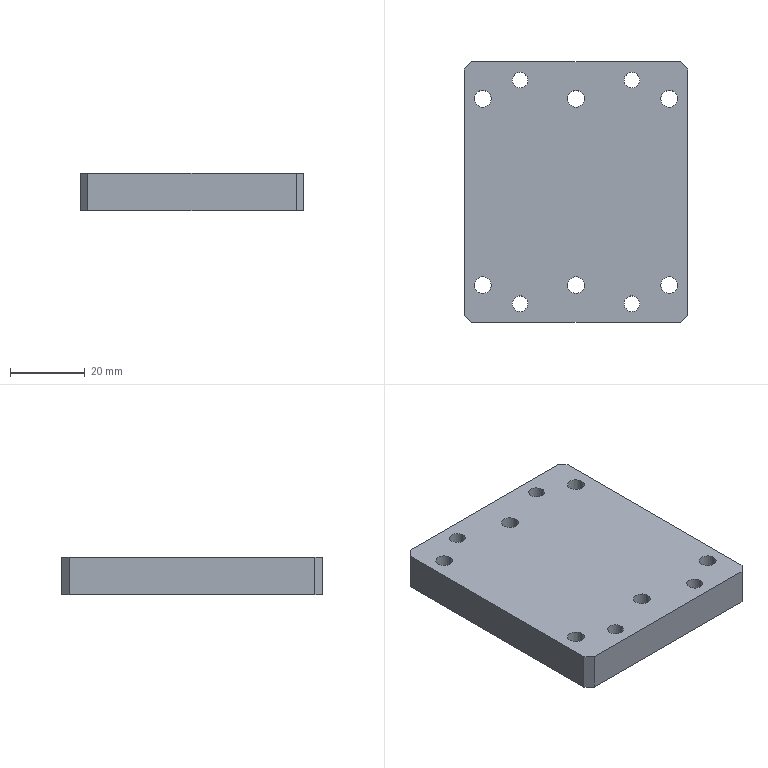Part | STEP file | 04-02-06 adjustment base plate | 1 solid | 48 faces | box 60 x 70 x 10 mm | volume 39504 mm3 | cylinder 32 | plane 16 | commonest cylinder face diameters 4.5 x12 8 x12 4.2 x8
STEP:
#1=CARTESIAN_POINT('',(12.9,-30.,10.));
#2=VERTEX_POINT('',#1);
#3=CARTESIAN_POINT('',(17.1,-30.,10.));
#4=VERTEX_POINT('',#3);
#5=CARTESIAN_POINT('',(15.,-30.,10.));
#6=DIRECTION('',(0.,0.,1.));
#7=DIRECTION('',(1.,0.,0.));
#8=AXIS2_PLACEMENT_3D('',#5,#6,#7);
#9=CIRCLE('',#8,2.1);
#10=EDGE_CURVE('',#2,#4,#9,.T.);
#11=ORIENTED_EDGE('',*,*,#10,.T.);
#12=CARTESIAN_POINT('',(17.1,-30.,0.));
#13=VERTEX_POINT('',#12);
#14=CARTESIAN_POINT('',(17.1,-30.,0.));
#15=DIRECTION('',(0.,0.,-1.));
#16=VECTOR('',#15,1000.);
#17=LINE('',#14,#16);
#18=EDGE_CURVE('',#4,#13,#17,.T.);
#19=ORIENTED_EDGE('',*,*,#18,.T.);
#20=CARTESIAN_POINT('',(12.9,-30.,0.));
#21=VERTEX_POINT('',#20);
#22=CARTESIAN_POINT('',(15.,-30.,0.));
#23=DIRECTION('',(0.,0.,-1.));
#24=DIRECTION('',(-1.,0.,0.));
#25=AXIS2_PLACEMENT_3D('',#22,#23,#24);
#26=CIRCLE('',#25,2.1);
#27=EDGE_CURVE('',#13,#21,#26,.T.);
#28=ORIENTED_EDGE('',*,*,#27,.T.);
#29=CARTESIAN_POINT('',(12.9,-30.,0.));
#30=DIRECTION('',(0.,0.,-1.));
#31=VECTOR('',#30,1000.);
#32=LINE('',#29,#31);
#33=EDGE_CURVE('',#2,#21,#32,.T.);
#34=ORIENTED_EDGE('',*,*,#33,.F.);
#35=EDGE_LOOP('',(#11,#19,#28,#34));
#36=FACE_OUTER_BOUND('',#35,.T.);
#37=CARTESIAN_POINT('',(15.,-30.,0.));
#38=DIRECTION('',(0.,0.,-1.));
#39=DIRECTION('',(-1.,0.,0.));
#40=AXIS2_PLACEMENT_3D('',#37,#38,#39);
#41=CYLINDRICAL_SURFACE('',#40,2.1);
#42=ADVANCED_FACE('',(#36),#41,.F.);
#43=CARTESIAN_POINT('',(12.9,30.,10.));
#44=VERTEX_POINT('',#43);
#45=CARTESIAN_POINT('',(17.1,30.,10.));
#46=VERTEX_POINT('',#45);
#47=CARTESIAN_POINT('',(15.,30.,10.));
#48=DIRECTION('',(0.,0.,1.));
#49=DIRECTION('',(1.,0.,0.));
#50=AXIS2_PLACEMENT_3D('',#47,#48,#49);
#51=CIRCLE('',#50,2.1);
#52=EDGE_CURVE('',#44,#46,#51,.T.);
#53=ORIENTED_EDGE('',*,*,#52,.T.);
#54=CARTESIAN_POINT('',(17.1,30.,0.));
#55=VERTEX_POINT('',#54);
#56=CARTESIAN_POINT('',(17.1,30.,0.));
#57=DIRECTION('',(0.,0.,-1.));
#58=VECTOR('',#57,1000.);
#59=LINE('',#56,#58);
#60=EDGE_CURVE('',#46,#55,#59,.T.);
#61=ORIENTED_EDGE('',*,*,#60,.T.);
#62=CARTESIAN_POINT('',(12.9,30.,0.));
#63=VERTEX_POINT('',#62);
#64=CARTESIAN_POINT('',(15.,30.,0.));
#65=DIRECTION('',(0.,0.,-1.));
#66=DIRECTION('',(-1.,0.,0.));
#67=AXIS2_PLACEMENT_3D('',#64,#65,#66);
#68=CIRCLE('',#67,2.1);
#69=EDGE_CURVE('',#55,#63,#68,.T.);
#70=ORIENTED_EDGE('',*,*,#69,.T.);
#71=CARTESIAN_POINT('',(12.9,30.,0.));
#72=DIRECTION('',(0.,0.,-1.));
#73=VECTOR('',#72,1000.);
#74=LINE('',#71,#73);
#75=EDGE_CURVE('',#44,#63,#74,.T.);
#76=ORIENTED_EDGE('',*,*,#75,.F.);
#77=EDGE_LOOP('',(#53,#61,#70,#76));
#78=FACE_OUTER_BOUND('',#77,.T.);
#79=CARTESIAN_POINT('',(15.,30.,0.));
#80=DIRECTION('',(0.,0.,-1.));
#81=DIRECTION('',(-1.,0.,0.));
#82=AXIS2_PLACEMENT_3D('',#79,#80,#81);
#83=CYLINDRICAL_SURFACE('',#82,2.1);
#84=ADVANCED_FACE('',(#78),#83,.F.);
#85=CARTESIAN_POINT('',(-17.1,30.,10.));
#86=VERTEX_POINT('',#85);
#87=CARTESIAN_POINT('',(-12.9,30.,10.));
#88=VERTEX_POINT('',#87);
#89=CARTESIAN_POINT('',(-15.,30.,10.));
#90=DIRECTION('',(0.,0.,1.));
#91=DIRECTION('',(1.,0.,0.));
#92=AXIS2_PLACEMENT_3D('',#89,#90,#91);
#93=CIRCLE('',#92,2.1);
#94=EDGE_CURVE('',#86,#88,#93,.T.);
#95=ORIENTED_EDGE('',*,*,#94,.T.);
#96=CARTESIAN_POINT('',(-12.9,30.,0.));
#97=VERTEX_POINT('',#96);
#98=CARTESIAN_POINT('',(-12.9,30.,0.));
#99=DIRECTION('',(0.,0.,-1.));
#100=VECTOR('',#99,1000.);
#101=LINE('',#98,#100);
#102=EDGE_CURVE('',#88,#97,#101,.T.);
#103=ORIENTED_EDGE('',*,*,#102,.T.);
#104=CARTESIAN_POINT('',(-17.1,30.,0.));
#105=VERTEX_POINT('',#104);
#106=CARTESIAN_POINT('',(-15.,30.,0.));
#107=DIRECTION('',(0.,0.,-1.));
#108=DIRECTION('',(-1.,0.,0.));
#109=AXIS2_PLACEMENT_3D('',#106,#107,#108);
#110=CIRCLE('',#109,2.1);
#111=EDGE_CURVE('',#97,#105,#110,.T.);
#112=ORIENTED_EDGE('',*,*,#111,.T.);
#113=CARTESIAN_POINT('',(-17.1,30.,0.));
#114=DIRECTION('',(0.,0.,-1.));
#115=VECTOR('',#114,1000.);
#116=LINE('',#113,#115);
#117=EDGE_CURVE('',#86,#105,#116,.T.);
#118=ORIENTED_EDGE('',*,*,#117,.F.);
#119=EDGE_LOOP('',(#95,#103,#112,#118));
#120=FACE_OUTER_BOUND('',#119,.T.);
#121=CARTESIAN_POINT('',(-15.,30.,0.));
#122=DIRECTION('',(0.,0.,-1.));
#123=DIRECTION('',(-1.,0.,0.));
#124=AXIS2_PLACEMENT_3D('',#121,#122,#123);
#125=CYLINDRICAL_SURFACE('',#124,2.1);
#126=ADVANCED_FACE('',(#120),#125,.F.);
#127=CARTESIAN_POINT('',(-17.1,-30.,10.));
#128=VERTEX_POINT('',#127);
#129=CARTESIAN_POINT('',(-12.9,-30.,10.));
#130=VERTEX_POINT('',#129);
#131=CARTESIAN_POINT('',(-15.,-30.,10.));
#132=DIRECTION('',(0.,0.,1.));
#133=DIRECTION('',(1.,0.,0.));
#134=AXIS2_PLACEMENT_3D('',#131,#132,#133);
#135=CIRCLE('',#134,2.1);
#136=EDGE_CURVE('',#128,#130,#135,.T.);
#137=ORIENTED_EDGE('',*,*,#136,.T.);
#138=CARTESIAN_POINT('',(-12.9,-30.,0.));
#139=VERTEX_POINT('',#138);
#140=CARTESIAN_POINT('',(-12.9,-30.,0.));
#141=DIRECTION('',(0.,0.,-1.));
#142=VECTOR('',#141,1000.);
#143=LINE('',#140,#142);
#144=EDGE_CURVE('',#130,#139,#143,.T.);
#145=ORIENTED_EDGE('',*,*,#144,.T.);
#146=CARTESIAN_POINT('',(-17.1,-30.,0.));
#147=VERTEX_POINT('',#146);
#148=CARTESIAN_POINT('',(-15.,-30.,0.));
#149=DIRECTION('',(0.,0.,-1.));
#150=DIRECTION('',(-1.,0.,0.));
#151=AXIS2_PLACEMENT_3D('',#148,#149,#150);
#152=CIRCLE('',#151,2.1);
#153=EDGE_CURVE('',#139,#147,#152,.T.);
#154=ORIENTED_EDGE('',*,*,#153,.T.);
#155=CARTESIAN_POINT('',(-17.1,-30.,0.));
#156=DIRECTION('',(0.,0.,-1.));
#157=VECTOR('',#156,1000.);
#158=LINE('',#155,#157);
#159=EDGE_CURVE('',#128,#147,#158,.T.);
#160=ORIENTED_EDGE('',*,*,#159,.F.);
#161=EDGE_LOOP('',(#137,#145,#154,#160));
#162=FACE_OUTER_BOUND('',#161,.T.);
#163=CARTESIAN_POINT('',(-15.,-30.,0.));
#164=DIRECTION('',(0.,0.,-1.));
#165=DIRECTION('',(-1.,0.,0.));
#166=AXIS2_PLACEMENT_3D('',#163,#164,#165);
#167=CYLINDRICAL_SURFACE('',#166,2.1);
#168=ADVANCED_FACE('',(#162),#167,.F.);
#169=CARTESIAN_POINT('',(29.,25.,4.4));
#170=VERTEX_POINT('',#169);
#171=CARTESIAN_POINT('',(21.,25.,4.4));
#172=VERTEX_POINT('',#171);
#173=CARTESIAN_POINT('',(25.,25.,4.4));
#174=DIRECTION('',(0.,0.,-1.));
#175=DIRECTION('',(-1.,0.,0.));
#176=AXIS2_PLACEMENT_3D('',#173,#174,#175);
#177=CIRCLE('',#176,4.);
#178=EDGE_CURVE('',#170,#172,#177,.T.);
#179=ORIENTED_EDGE('',*,*,#178,.F.);
#180=CARTESIAN_POINT('',(29.,25.,0.));
#181=VERTEX_POINT('',#180);
#182=CARTESIAN_POINT('',(29.,25.,0.));
#183=DIRECTION('',(0.,0.,-1.));
#184=VECTOR('',#183,1000.);
#185=LINE('',#182,#184);
#186=EDGE_CURVE('',#170,#181,#185,.T.);
#187=ORIENTED_EDGE('',*,*,#186,.T.);
#188=CARTESIAN_POINT('',(21.,25.,0.));
#189=VERTEX_POINT('',#188);
#190=CARTESIAN_POINT('',(25.,25.,0.));
#191=DIRECTION('',(0.,0.,-1.));
#192=DIRECTION('',(-1.,0.,0.));
#193=AXIS2_PLACEMENT_3D('',#190,#191,#192);
#194=CIRCLE('',#193,4.);
#195=EDGE_CURVE('',#181,#189,#194,.T.);
#196=ORIENTED_EDGE('',*,*,#195,.T.);
#197=CARTESIAN_POINT('',(21.,25.,0.));
#198=DIRECTION('',(0.,0.,-1.));
#199=VECTOR('',#198,1000.);
#200=LINE('',#197,#199);
#201=EDGE_CURVE('',#172,#189,#200,.T.);
#202=ORIENTED_EDGE('',*,*,#201,.F.);
#203=EDGE_LOOP('',(#179,#187,#196,#202));
#204=FACE_OUTER_BOUND('',#203,.T.);
#205=CARTESIAN_POINT('',(25.,25.,0.));
#206=DIRECTION('',(0.,0.,-1.));
#207=DIRECTION('',(-1.,0.,0.));
#208=AXIS2_PLACEMENT_3D('',#205,#206,#207);
#209=CYLINDRICAL_SURFACE('',#208,4.);
#210=ADVANCED_FACE('',(#204),#209,.F.);
#211=CARTESIAN_POINT('',(27.25,25.,10.));
#212=VERTEX_POINT('',#211);
#213=CARTESIAN_POINT('',(22.75,25.,10.));
#214=VERTEX_POINT('',#213);
#215=CARTESIAN_POINT('',(25.,25.,10.));
#216=DIRECTION('',(0.,0.,-1.));
#217=DIRECTION('',(-1.,0.,0.));
#218=AXIS2_PLACEMENT_3D('',#215,#216,#217);
#219=CIRCLE('',#218,2.25);
#220=EDGE_CURVE('',#212,#214,#219,.T.);
#221=ORIENTED_EDGE('',*,*,#220,.F.);
#222=CARTESIAN_POINT('',(27.25,25.,4.4));
#223=VERTEX_POINT('',#222);
#224=CARTESIAN_POINT('',(27.25,25.,0.));
#225=DIRECTION('',(0.,0.,-1.));
#226=VECTOR('',#225,1000.);
#227=LINE('',#224,#226);
#228=EDGE_CURVE('',#212,#223,#227,.T.);
#229=ORIENTED_EDGE('',*,*,#228,.T.);
#230=CARTESIAN_POINT('',(22.75,25.,4.4));
#231=VERTEX_POINT('',#230);
#232=CARTESIAN_POINT('',(25.,25.,4.4));
#233=DIRECTION('',(0.,0.,-1.));
#234=DIRECTION('',(-1.,0.,0.));
#235=AXIS2_PLACEMENT_3D('',#232,#233,#234);
#236=CIRCLE('',#235,2.25);
#237=EDGE_CURVE('',#223,#231,#236,.T.);
#238=ORIENTED_EDGE('',*,*,#237,.T.);
#239=CARTESIAN_POINT('',(22.75,25.,0.));
#240=DIRECTION('',(0.,0.,-1.));
#241=VECTOR('',#240,1000.);
#242=LINE('',#239,#241);
#243=EDGE_CURVE('',#214,#231,#242,.T.);
#244=ORIENTED_EDGE('',*,*,#243,.F.);
#245=EDGE_LOOP('',(#221,#229,#238,#244));
#246=FACE_OUTER_BOUND('',#245,.T.);
#247=CARTESIAN_POINT('',(25.,25.,0.));
#248=DIRECTION('',(0.,0.,-1.));
#249=DIRECTION('',(-1.,0.,0.));
#250=AXIS2_PLACEMENT_3D('',#247,#248,#249);
#251=CYLINDRICAL_SURFACE('',#250,2.25);
#252=ADVANCED_FACE('',(#246),#251,.F.);
#253=CARTESIAN_POINT('',(29.,-25.,4.4));
#254=VERTEX_POINT('',#253);
#255=CARTESIAN_POINT('',(21.,-25.,4.4));
#256=VERTEX_POINT('',#255);
#257=CARTESIAN_POINT('',(25.,-25.,4.4));
#258=DIRECTION('',(0.,0.,-1.));
#259=DIRECTION('',(-1.,0.,0.));
#260=AXIS2_PLACEMENT_3D('',#257,#258,#259);
#261=CIRCLE('',#260,4.);
#262=EDGE_CURVE('',#254,#256,#261,.T.);
#263=ORIENTED_EDGE('',*,*,#262,.F.);
#264=CARTESIAN_POINT('',(29.,-25.,0.));
#265=VERTEX_POINT('',#264);
#266=CARTESIAN_POINT('',(29.,-25.,0.));
#267=DIRECTION('',(0.,0.,-1.));
#268=VECTOR('',#267,1000.);
#269=LINE('',#266,#268);
#270=EDGE_CURVE('',#254,#265,#269,.T.);
#271=ORIENTED_EDGE('',*,*,#270,.T.);
#272=CARTESIAN_POINT('',(21.,-25.,0.));
#273=VERTEX_POINT('',#272);
#274=CARTESIAN_POINT('',(25.,-25.,0.));
#275=DIRECTION('',(0.,0.,-1.));
#276=DIRECTION('',(-1.,0.,0.));
#277=AXIS2_PLACEMENT_3D('',#274,#275,#276);
#278=CIRCLE('',#277,4.);
#279=EDGE_CURVE('',#265,#273,#278,.T.);
#280=ORIENTED_EDGE('',*,*,#279,.T.);
#281=CARTESIAN_POINT('',(21.,-25.,0.));
#282=DIRECTION('',(0.,0.,-1.));
#283=VECTOR('',#282,1000.);
#284=LINE('',#281,#283);
#285=EDGE_CURVE('',#256,#273,#284,.T.);
#286=ORIENTED_EDGE('',*,*,#285,.F.);
#287=EDGE_LOOP('',(#263,#271,#280,#286));
#288=FACE_OUTER_BOUND('',#287,.T.);
#289=CARTESIAN_POINT('',(25.,-25.,0.));
#290=DIRECTION('',(0.,0.,-1.));
#291=DIRECTION('',(-1.,0.,0.));
#292=AXIS2_PLACEMENT_3D('',#289,#290,#291);
#293=CYLINDRICAL_SURFACE('',#292,4.);
#294=ADVANCED_FACE('',(#288),#293,.F.);
#295=CARTESIAN_POINT('',(27.25,-25.,10.));
#296=VERTEX_POINT('',#295);
#297=CARTESIAN_POINT('',(22.75,-25.,10.));
#298=VERTEX_POINT('',#297);
#299=CARTESIAN_POINT('',(25.,-25.,10.));
#300=DIRECTION('',(0.,0.,-1.));
#301=DIRECTION('',(-1.,0.,0.));
#302=AXIS2_PLACEMENT_3D('',#299,#300,#301);
#303=CIRCLE('',#302,2.25);
#304=EDGE_CURVE('',#296,#298,#303,.T.);
#305=ORIENTED_EDGE('',*,*,#304,.F.);
#306=CARTESIAN_POINT('',(27.25,-25.,4.4));
#307=VERTEX_POINT('',#306);
#308=CARTESIAN_POINT('',(27.25,-25.,0.));
#309=DIRECTION('',(0.,0.,-1.));
#310=VECTOR('',#309,1000.);
#311=LINE('',#308,#310);
#312=EDGE_CURVE('',#296,#307,#311,.T.);
#313=ORIENTED_EDGE('',*,*,#312,.T.);
#314=CARTESIAN_POINT('',(22.75,-25.,4.4));
#315=VERTEX_POINT('',#314);
#316=CARTESIAN_POINT('',(25.,-25.,4.4));
#317=DIRECTION('',(0.,0.,-1.));
#318=DIRECTION('',(-1.,0.,0.));
#319=AXIS2_PLACEMENT_3D('',#316,#317,#318);
#320=CIRCLE('',#319,2.25);
#321=EDGE_CURVE('',#307,#315,#320,.T.);
#322=ORIENTED_EDGE('',*,*,#321,.T.);
#323=CARTESIAN_POINT('',(22.75,-25.,0.));
#324=DIRECTION('',(0.,0.,-1.));
#325=VECTOR('',#324,1000.);
#326=LINE('',#323,#325);
#327=EDGE_CURVE('',#298,#315,#326,.T.);
#328=ORIENTED_EDGE('',*,*,#327,.F.);
#329=EDGE_LOOP('',(#305,#313,#322,#328));
#330=FACE_OUTER_BOUND('',#329,.T.);
#331=CARTESIAN_POINT('',(25.,-25.,0.));
#332=DIRECTION('',(0.,0.,-1.));
#333=DIRECTION('',(-1.,0.,0.));
#334=AXIS2_PLACEMENT_3D('',#331,#332,#333);
#335=CYLINDRICAL_SURFACE('',#334,2.25);
#336=ADVANCED_FACE('',(#330),#335,.F.);
#337=CARTESIAN_POINT('',(4.,-25.,4.4));
#338=VERTEX_POINT('',#337);
#339=CARTESIAN_POINT('',(-4.,-25.,4.4));
#340=VERTEX_POINT('',#339);
#341=CARTESIAN_POINT('',(0.,-25.,4.4));
#342=DIRECTION('',(0.,0.,-1.));
#343=DIRECTION('',(-1.,0.,0.));
#344=AXIS2_PLACEMENT_3D('',#341,#342,#343);
#345=CIRCLE('',#344,4.);
#346=EDGE_CURVE('',#338,#340,#345,.T.);
#347=ORIENTED_EDGE('',*,*,#346,.F.);
#348=CARTESIAN_POINT('',(4.,-25.,0.));
#349=VERTEX_POINT('',#348);
#350=CARTESIAN_POINT('',(4.,-25.,0.));
#351=DIRECTION('',(0.,0.,-1.));
#352=VECTOR('',#351,1000.);
#353=LINE('',#350,#352);
#354=EDGE_CURVE('',#338,#349,#353,.T.);
#355=ORIENTED_EDGE('',*,*,#354,.T.);
#356=CARTESIAN_POINT('',(-4.,-25.,0.));
#357=VERTEX_POINT('',#356);
#358=CARTESIAN_POINT('',(0.,-25.,0.));
#359=DIRECTION('',(0.,0.,-1.));
#360=DIRECTION('',(-1.,0.,0.));
#361=AXIS2_PLACEMENT_3D('',#358,#359,#360);
#362=CIRCLE('',#361,4.);
#363=EDGE_CURVE('',#349,#357,#362,.T.);
#364=ORIENTED_EDGE('',*,*,#363,.T.);
#365=CARTESIAN_POINT('',(-4.,-25.,0.));
#366=DIRECTION('',(0.,0.,-1.));
#367=VECTOR('',#366,1000.);
#368=LINE('',#365,#367);
#369=EDGE_CURVE('',#340,#357,#368,.T.);
#370=ORIENTED_EDGE('',*,*,#369,.F.);
#371=EDGE_LOOP('',(#347,#355,#364,#370));
#372=FACE_OUTER_BOUND('',#371,.T.);
#373=CARTESIAN_POINT('',(0.,-25.,0.));
#374=DIRECTION('',(0.,0.,-1.));
#375=DIRECTION('',(-1.,0.,0.));
#376=AXIS2_PLACEMENT_3D('',#373,#374,#375);
#377=CYLINDRICAL_SURFACE('',#376,4.);
#378=ADVANCED_FACE('',(#372),#377,.F.);
#379=CARTESIAN_POINT('',(2.25,-25.,10.));
#380=VERTEX_POINT('',#379);
#381=CARTESIAN_POINT('',(-2.25,-25.,10.));
#382=VERTEX_POINT('',#381);
#383=CARTESIAN_POINT('',(0.,-25.,10.));
#384=DIRECTION('',(0.,0.,-1.));
#385=DIRECTION('',(-1.,0.,0.));
#386=AXIS2_PLACEMENT_3D('',#383,#384,#385);
#387=CIRCLE('',#386,2.25);
#388=EDGE_CURVE('',#380,#382,#387,.T.);
#389=ORIENTED_EDGE('',*,*,#388,.F.);
#390=CARTESIAN_POINT('',(2.25,-25.,4.4));
#391=VERTEX_POINT('',#390);
#392=CARTESIAN_POINT('',(2.25,-25.,0.));
#393=DIRECTION('',(0.,0.,-1.));
#394=VECTOR('',#393,1000.);
#395=LINE('',#392,#394);
#396=EDGE_CURVE('',#380,#391,#395,.T.);
#397=ORIENTED_EDGE('',*,*,#396,.T.);
#398=CARTESIAN_POINT('',(-2.25,-25.,4.4));
#399=VERTEX_POINT('',#398);
#400=CARTESIAN_POINT('',(0.,-25.,4.4));
#401=DIRECTION('',(0.,0.,-1.));
#402=DIRECTION('',(-1.,0.,0.));
#403=AXIS2_PLACEMENT_3D('',#400,#401,#402);
#404=CIRCLE('',#403,2.25);
#405=EDGE_CURVE('',#391,#399,#404,.T.);
#406=ORIENTED_EDGE('',*,*,#405,.T.);
#407=CARTESIAN_POINT('',(-2.25,-25.,0.));
#408=DIRECTION('',(0.,0.,-1.));
#409=VECTOR('',#408,1000.);
#410=LINE('',#407,#409);
#411=EDGE_CURVE('',#382,#399,#410,.T.);
#412=ORIENTED_EDGE('',*,*,#411,.F.);
#413=EDGE_LOOP('',(#389,#397,#406,#412));
#414=FACE_OUTER_BOUND('',#413,.T.);
#415=CARTESIAN_POINT('',(0.,-25.,0.));
#416=DIRECTION('',(0.,0.,-1.));
#417=DIRECTION('',(-1.,0.,0.));
#418=AXIS2_PLACEMENT_3D('',#415,#416,#417);
#419=CYLINDRICAL_SURFACE('',#418,2.25);
#420=ADVANCED_FACE('',(#414),#419,.F.);
#421=CARTESIAN_POINT('',(-21.,-25.,4.4));
#422=VERTEX_POINT('',#421);
#423=CARTESIAN_POINT('',(-29.,-25.,4.4));
#424=VERTEX_POINT('',#423);
#425=CARTESIAN_POINT('',(-25.,-25.,4.4));
#426=DIRECTION('',(0.,0.,-1.));
#427=DIRECTION('',(-1.,0.,0.));
#428=AXIS2_PLACEMENT_3D('',#425,#426,#427);
#429=CIRCLE('',#428,4.);
#430=EDGE_CURVE('',#422,#424,#429,.T.);
#431=ORIENTED_EDGE('',*,*,#430,.F.);
#432=CARTESIAN_POINT('',(-21.,-25.,0.));
#433=VERTEX_POINT('',#432);
#434=CARTESIAN_POINT('',(-21.,-25.,0.));
#435=DIRECTION('',(0.,0.,-1.));
#436=VECTOR('',#435,1000.);
#437=LINE('',#434,#436);
#438=EDGE_CURVE('',#422,#433,#437,.T.);
#439=ORIENTED_EDGE('',*,*,#438,.T.);
#440=CARTESIAN_POINT('',(-29.,-25.,0.));
#441=VERTEX_POINT('',#440);
#442=CARTESIAN_POINT('',(-25.,-25.,0.));
#443=DIRECTION('',(0.,0.,-1.));
#444=DIRECTION('',(-1.,0.,0.));
#445=AXIS2_PLACEMENT_3D('',#442,#443,#444);
#446=CIRCLE('',#445,4.);
#447=EDGE_CURVE('',#433,#441,#446,.T.);
#448=ORIENTED_EDGE('',*,*,#447,.T.);
#449=CARTESIAN_POINT('',(-29.,-25.,0.));
#450=DIRECTION('',(0.,0.,-1.));
#451=VECTOR('',#450,1000.);
#452=LINE('',#449,#451);
#453=EDGE_CURVE('',#424,#441,#452,.T.);
#454=ORIENTED_EDGE('',*,*,#453,.F.);
#455=EDGE_LOOP('',(#431,#439,#448,#454));
#456=FACE_OUTER_BOUND('',#455,.T.);
#457=CARTESIAN_POINT('',(-25.,-25.,0.));
#458=DIRECTION('',(0.,0.,-1.));
#459=DIRECTION('',(-1.,0.,0.));
#460=AXIS2_PLACEMENT_3D('',#457,#458,#459);
#461=CYLINDRICAL_SURFACE('',#460,4.);
#462=ADVANCED_FACE('',(#456),#461,.F.);
#463=CARTESIAN_POINT('',(-22.75,-25.,10.));
#464=VERTEX_POINT('',#463);
#465=CARTESIAN_POINT('',(-27.25,-25.,10.));
#466=VERTEX_POINT('',#465);
#467=CARTESIAN_POINT('',(-25.,-25.,10.));
#468=DIRECTION('',(0.,0.,-1.));
#469=DIRECTION('',(-1.,0.,0.));
#470=AXIS2_PLACEMENT_3D('',#467,#468,#469);
#471=CIRCLE('',#470,2.25);
#472=EDGE_CURVE('',#464,#466,#471,.T.);
#473=ORIENTED_EDGE('',*,*,#472,.F.);
#474=CARTESIAN_POINT('',(-22.75,-25.,4.4));
#475=VERTEX_POINT('',#474);
#476=CARTESIAN_POINT('',(-22.75,-25.,0.));
#477=DIRECTION('',(0.,0.,-1.));
#478=VECTOR('',#477,1000.);
#479=LINE('',#476,#478);
#480=EDGE_CURVE('',#464,#475,#479,.T.);
#481=ORIENTED_EDGE('',*,*,#480,.T.);
#482=CARTESIAN_POINT('',(-27.25,-25.,4.4));
#483=VERTEX_POINT('',#482);
#484=CARTESIAN_POINT('',(-25.,-25.,4.4));
#485=DIRECTION('',(0.,0.,-1.));
#486=DIRECTION('',(-1.,0.,0.));
#487=AXIS2_PLACEMENT_3D('',#484,#485,#486);
#488=CIRCLE('',#487,2.25);
#489=EDGE_CURVE('',#475,#483,#488,.T.);
#490=ORIENTED_EDGE('',*,*,#489,.T.);
#491=CARTESIAN_POINT('',(-27.25,-25.,0.));
#492=DIRECTION('',(0.,0.,-1.));
#493=VECTOR('',#492,1000.);
#494=LINE('',#491,#493);
#495=EDGE_CURVE('',#466,#483,#494,.T.);
#496=ORIENTED_EDGE('',*,*,#495,.F.);
#497=EDGE_LOOP('',(#473,#481,#490,#496));
#498=FACE_OUTER_BOUND('',#497,.T.);
#499=CARTESIAN_POINT('',(-25.,-25.,0.));
#500=DIRECTION('',(0.,0.,-1.));
#501=DIRECTION('',(-1.,0.,0.));
#502=AXIS2_PLACEMENT_3D('',#499,#500,#501);
#503=CYLINDRICAL_SURFACE('',#502,2.25);
#504=ADVANCED_FACE('',(#498),#503,.F.);
#505=CARTESIAN_POINT('',(-21.,25.,4.4));
#506=VERTEX_POINT('',#505);
#507=CARTESIAN_POINT('',(-29.,25.,4.4));
#508=VERTEX_POINT('',#507);
#509=CARTESIAN_POINT('',(-25.,25.,4.4));
#510=DIRECTION('',(0.,0.,-1.));
#511=DIRECTION('',(-1.,0.,0.));
#512=AXIS2_PLACEMENT_3D('',#509,#510,#511);
#513=CIRCLE('',#512,4.);
#514=EDGE_CURVE('',#506,#508,#513,.T.);
#515=ORIENTED_EDGE('',*,*,#514,.F.);
#516=CARTESIAN_POINT('',(-21.,25.,0.));
#517=VERTEX_POINT('',#516);
#518=CARTESIAN_POINT('',(-21.,25.,0.));
#519=DIRECTION('',(0.,0.,-1.));
#520=VECTOR('',#519,1000.);
#521=LINE('',#518,#520);
#522=EDGE_CURVE('',#506,#517,#521,.T.);
#523=ORIENTED_EDGE('',*,*,#522,.T.);
#524=CARTESIAN_POINT('',(-29.,25.,0.));
#525=VERTEX_POINT('',#524);
#526=CARTESIAN_POINT('',(-25.,25.,0.));
#527=DIRECTION('',(0.,0.,-1.));
#528=DIRECTION('',(-1.,0.,0.));
#529=AXIS2_PLACEMENT_3D('',#526,#527,#528);
#530=CIRCLE('',#529,4.);
#531=EDGE_CURVE('',#517,#525,#530,.T.);
#532=ORIENTED_EDGE('',*,*,#531,.T.);
#533=CARTESIAN_POINT('',(-29.,25.,0.));
#534=DIRECTION('',(0.,0.,-1.));
#535=VECTOR('',#534,1000.);
#536=LINE('',#533,#535);
#537=EDGE_CURVE('',#508,#525,#536,.T.);
#538=ORIENTED_EDGE('',*,*,#537,.F.);
#539=EDGE_LOOP('',(#515,#523,#532,#538));
#540=FACE_OUTER_BOUND('',#539,.T.);
#541=CARTESIAN_POINT('',(-25.,25.,0.));
#542=DIRECTION('',(0.,0.,-1.));
#543=DIRECTION('',(-1.,0.,0.));
#544=AXIS2_PLACEMENT_3D('',#541,#542,#543);
#545=CYLINDRICAL_SURFACE('',#544,4.);
#546=ADVANCED_FACE('',(#540),#545,.F.);
#547=CARTESIAN_POINT('',(-22.75,25.,10.));
#548=VERTEX_POINT('',#547);
#549=CARTESIAN_POINT('',(-27.25,25.,10.));
#550=VERTEX_POINT('',#549);
#551=CARTESIAN_POINT('',(-25.,25.,10.));
#552=DIRECTION('',(0.,0.,-1.));
#553=DIRECTION('',(-1.,0.,0.));
#554=AXIS2_PLACEMENT_3D('',#551,#552,#553);
#555=CIRCLE('',#554,2.25);
#556=EDGE_CURVE('',#548,#550,#555,.T.);
#557=ORIENTED_EDGE('',*,*,#556,.F.);
#558=CARTESIAN_POINT('',(-22.75,25.,4.4));
#559=VERTEX_POINT('',#558);
#560=CARTESIAN_POINT('',(-22.75,25.,0.));
#561=DIRECTION('',(0.,0.,-1.));
#562=VECTOR('',#561,1000.);
#563=LINE('',#560,#562);
#564=EDGE_CURVE('',#548,#559,#563,.T.);
#565=ORIENTED_EDGE('',*,*,#564,.T.);
#566=CARTESIAN_POINT('',(-27.25,25.,4.4));
#567=VERTEX_POINT('',#566);
#568=CARTESIAN_POINT('',(-25.,25.,4.4));
#569=DIRECTION('',(0.,0.,-1.));
#570=DIRECTION('',(-1.,0.,0.));
#571=AXIS2_PLACEMENT_3D('',#568,#569,#570);
#572=CIRCLE('',#571,2.25);
#573=EDGE_CURVE('',#559,#567,#572,.T.);
#574=ORIENTED_EDGE('',*,*,#573,.T.);
#575=CARTESIAN_POINT('',(-27.25,25.,0.));
#576=DIRECTION('',(0.,0.,-1.));
#577=VECTOR('',#576,1000.);
#578=LINE('',#575,#577);
#579=EDGE_CURVE('',#550,#567,#578,.T.);
#580=ORIENTED_EDGE('',*,*,#579,.F.);
#581=EDGE_LOOP('',(#557,#565,#574,#580));
#582=FACE_OUTER_BOUND('',#581,.T.);
#583=CARTESIAN_POINT('',(-25.,25.,0.));
#584=DIRECTION('',(0.,0.,-1.));
#585=DIRECTION('',(-1.,0.,0.));
#586=AXIS2_PLACEMENT_3D('',#583,#584,#585);
#587=CYLINDRICAL_SURFACE('',#586,2.25);
#588=ADVANCED_FACE('',(#582),#587,.F.);
#589=CARTESIAN_POINT('',(4.,25.,4.4));
#590=VERTEX_POINT('',#589);
#591=CARTESIAN_POINT('',(-4.,25.,4.4));
#592=VERTEX_POINT('',#591);
#593=CARTESIAN_POINT('',(0.,25.,4.4));
#594=DIRECTION('',(0.,0.,-1.));
#595=DIRECTION('',(-1.,0.,0.));
#596=AXIS2_PLACEMENT_3D('',#593,#594,#595);
#597=CIRCLE('',#596,4.);
#598=EDGE_CURVE('',#590,#592,#597,.T.);
#599=ORIENTED_EDGE('',*,*,#598,.F.);
#600=CARTESIAN_POINT('',(4.,25.,0.));
#601=VERTEX_POINT('',#600);
#602=CARTESIAN_POINT('',(4.,25.,0.));
#603=DIRECTION('',(0.,0.,-1.));
#604=VECTOR('',#603,1000.);
#605=LINE('',#602,#604);
#606=EDGE_CURVE('',#590,#601,#605,.T.);
#607=ORIENTED_EDGE('',*,*,#606,.T.);
#608=CARTESIAN_POINT('',(-4.,25.,0.));
#609=VERTEX_POINT('',#608);
#610=CARTESIAN_POINT('',(0.,25.,0.));
#611=DIRECTION('',(0.,0.,-1.));
#612=DIRECTION('',(-1.,0.,0.));
#613=AXIS2_PLACEMENT_3D('',#610,#611,#612);
#614=CIRCLE('',#613,4.);
#615=EDGE_CURVE('',#601,#609,#614,.T.);
#616=ORIENTED_EDGE('',*,*,#615,.T.);
#617=CARTESIAN_POINT('',(-4.,25.,0.));
#618=DIRECTION('',(0.,0.,-1.));
#619=VECTOR('',#618,1000.);
#620=LINE('',#617,#619);
#621=EDGE_CURVE('',#592,#609,#620,.T.);
#622=ORIENTED_EDGE('',*,*,#621,.F.);
#623=EDGE_LOOP('',(#599,#607,#616,#622));
#624=FACE_OUTER_BOUND('',#623,.T.);
#625=CARTESIAN_POINT('',(0.,25.,0.));
#626=DIRECTION('',(0.,0.,-1.));
#627=DIRECTION('',(-1.,0.,0.));
#628=AXIS2_PLACEMENT_3D('',#625,#626,#627);
#629=CYLINDRICAL_SURFACE('',#628,4.);
#630=ADVANCED_FACE('',(#624),#629,.F.);
#631=CARTESIAN_POINT('',(2.25,25.,10.));
#632=VERTEX_POINT('',#631);
#633=CARTESIAN_POINT('',(-2.25,25.,10.));
#634=VERTEX_POINT('',#633);
#635=CARTESIAN_POINT('',(0.,25.,10.));
#636=DIRECTION('',(0.,0.,-1.));
#637=DIRECTION('',(-1.,0.,0.));
#638=AXIS2_PLACEMENT_3D('',#635,#636,#637);
#639=CIRCLE('',#638,2.25);
#640=EDGE_CURVE('',#632,#634,#639,.T.);
#641=ORIENTED_EDGE('',*,*,#640,.F.);
#642=CARTESIAN_POINT('',(2.25,25.,4.4));
#643=VERTEX_POINT('',#642);
#644=CARTESIAN_POINT('',(2.25,25.,0.));
#645=DIRECTION('',(0.,0.,-1.));
#646=VECTOR('',#645,1000.);
#647=LINE('',#644,#646);
#648=EDGE_CURVE('',#632,#643,#647,.T.);
#649=ORIENTED_EDGE('',*,*,#648,.T.);
#650=CARTESIAN_POINT('',(-2.25,25.,4.4));
#651=VERTEX_POINT('',#650);
#652=CARTESIAN_POINT('',(0.,25.,4.4));
#653=DIRECTION('',(0.,0.,-1.));
#654=DIRECTION('',(-1.,0.,0.));
#655=AXIS2_PLACEMENT_3D('',#652,#653,#654);
#656=CIRCLE('',#655,2.25);
#657=EDGE_CURVE('',#643,#651,#656,.T.);
#658=ORIENTED_EDGE('',*,*,#657,.T.);
#659=CARTESIAN_POINT('',(-2.25,25.,0.));
#660=DIRECTION('',(0.,0.,-1.));
#661=VECTOR('',#660,1000.);
#662=LINE('',#659,#661);
#663=EDGE_CURVE('',#634,#651,#662,.T.);
#664=ORIENTED_EDGE('',*,*,#663,.F.);
#665=EDGE_LOOP('',(#641,#649,#658,#664));
#666=FACE_OUTER_BOUND('',#665,.T.);
#667=CARTESIAN_POINT('',(0.,25.,0.));
#668=DIRECTION('',(0.,0.,-1.));
#669=DIRECTION('',(-1.,0.,0.));
#670=AXIS2_PLACEMENT_3D('',#667,#668,#669);
#671=CYLINDRICAL_SURFACE('',#670,2.25);
#672=ADVANCED_FACE('',(#666),#671,.F.);
#673=CARTESIAN_POINT('',(28.,35.,0.));
#674=VERTEX_POINT('',#673);
#675=CARTESIAN_POINT('',(-28.,35.,0.));
#676=VERTEX_POINT('',#675);
#677=CARTESIAN_POINT('',(-30.,35.,0.));
#678=DIRECTION('',(-1.,0.,0.));
#679=VECTOR('',#678,1000.);
#680=LINE('',#677,#679);
#681=EDGE_CURVE('',#674,#676,#680,.T.);
#682=ORIENTED_EDGE('',*,*,#681,.F.);
#683=CARTESIAN_POINT('',(30.,33.,0.));
#684=VERTEX_POINT('',#683);
#685=CARTESIAN_POINT('',(28.,35.,0.));
#686=DIRECTION('',(0.7071,-0.7071,0.));
#687=VECTOR('',#686,1000.);
#688=LINE('',#685,#687);
#689=EDGE_CURVE('',#674,#684,#688,.T.);
#690=ORIENTED_EDGE('',*,*,#689,.T.);
#691=CARTESIAN_POINT('',(30.,-33.,0.));
#692=VERTEX_POINT('',#691);
#693=CARTESIAN_POINT('',(30.,35.,0.));
#694=DIRECTION('',(0.,1.,0.));
#695=VECTOR('',#694,1000.);
#696=LINE('',#693,#695);
#697=EDGE_CURVE('',#692,#684,#696,.T.);
#698=ORIENTED_EDGE('',*,*,#697,.F.);
#699=CARTESIAN_POINT('',(28.,-35.,0.));
#700=VERTEX_POINT('',#699);
#701=CARTESIAN_POINT('',(30.,-33.,0.));
#702=DIRECTION('',(-0.7071,-0.7071,0.));
#703=VECTOR('',#702,1000.);
#704=LINE('',#701,#703);
#705=EDGE_CURVE('',#692,#700,#704,.T.);
#706=ORIENTED_EDGE('',*,*,#705,.T.);
#707=CARTESIAN_POINT('',(-28.,-35.,0.));
#708=VERTEX_POINT('',#707);
#709=CARTESIAN_POINT('',(-30.,-35.,0.));
#710=DIRECTION('',(1.,0.,0.));
#711=VECTOR('',#710,1000.);
#712=LINE('',#709,#711);
#713=EDGE_CURVE('',#708,#700,#712,.T.);
#714=ORIENTED_EDGE('',*,*,#713,.F.);
#715=CARTESIAN_POINT('',(-30.,-33.,0.));
#716=VERTEX_POINT('',#715);
#717=CARTESIAN_POINT('',(-28.,-35.,0.));
#718=DIRECTION('',(-0.7071,0.7071,0.));
#719=VECTOR('',#718,1000.);
#720=LINE('',#717,#719);
#721=EDGE_CURVE('',#708,#716,#720,.T.);
#722=ORIENTED_EDGE('',*,*,#721,.T.);
#723=CARTESIAN_POINT('',(-30.,33.,0.));
#724=VERTEX_POINT('',#723);
#725=CARTESIAN_POINT('',(-30.,35.,0.));
#726=DIRECTION('',(0.,-1.,0.));
#727=VECTOR('',#726,1000.);
#728=LINE('',#725,#727);
#729=EDGE_CURVE('',#724,#716,#728,.T.);
#730=ORIENTED_EDGE('',*,*,#729,.F.);
#731=CARTESIAN_POINT('',(-30.,33.,0.));
#732=DIRECTION('',(0.7071,0.7071,0.));
#733=VECTOR('',#732,1000.);
#734=LINE('',#731,#733);
#735=EDGE_CURVE('',#724,#676,#734,.T.);
#736=ORIENTED_EDGE('',*,*,#735,.T.);
#737=EDGE_LOOP('',(#682,#690,#698,#706,#714,#722,#730,#736));
#738=FACE_OUTER_BOUND('',#737,.T.);
#739=CARTESIAN_POINT('',(0.,25.,0.));
#740=DIRECTION('',(0.,0.,-1.));
#741=DIRECTION('',(-1.,0.,0.));
#742=AXIS2_PLACEMENT_3D('',#739,#740,#741);
#743=CIRCLE('',#742,4.);
#744=EDGE_CURVE('',#609,#601,#743,.T.);
#745=ORIENTED_EDGE('',*,*,#744,.F.);
#746=ORIENTED_EDGE('',*,*,#615,.F.);
#747=EDGE_LOOP('',(#745,#746));
#748=FACE_BOUND('',#747,.T.);
#749=CARTESIAN_POINT('',(-25.,25.,0.));
#750=DIRECTION('',(0.,0.,-1.));
#751=DIRECTION('',(-1.,0.,0.));
#752=AXIS2_PLACEMENT_3D('',#749,#750,#751);
#753=CIRCLE('',#752,4.);
#754=EDGE_CURVE('',#525,#517,#753,.T.);
#755=ORIENTED_EDGE('',*,*,#754,.F.);
#756=ORIENTED_EDGE('',*,*,#531,.F.);
#757=EDGE_LOOP('',(#755,#756));
#758=FACE_BOUND('',#757,.T.);
#759=CARTESIAN_POINT('',(-25.,-25.,0.));
#760=DIRECTION('',(0.,0.,-1.));
#761=DIRECTION('',(-1.,0.,0.));
#762=AXIS2_PLACEMENT_3D('',#759,#760,#761);
#763=CIRCLE('',#762,4.);
#764=EDGE_CURVE('',#441,#433,#763,.T.);
#765=ORIENTED_EDGE('',*,*,#764,.F.);
#766=ORIENTED_EDGE('',*,*,#447,.F.);
#767=EDGE_LOOP('',(#765,#766));
#768=FACE_BOUND('',#767,.T.);
#769=CARTESIAN_POINT('',(0.,-25.,0.));
#770=DIRECTION('',(0.,0.,-1.));
#771=DIRECTION('',(-1.,0.,0.));
#772=AXIS2_PLACEMENT_3D('',#769,#770,#771);
#773=CIRCLE('',#772,4.);
#774=EDGE_CURVE('',#357,#349,#773,.T.);
#775=ORIENTED_EDGE('',*,*,#774,.F.);
#776=ORIENTED_EDGE('',*,*,#363,.F.);
#777=EDGE_LOOP('',(#775,#776));
#778=FACE_BOUND('',#777,.T.);
#779=CARTESIAN_POINT('',(25.,-25.,0.));
#780=DIRECTION('',(0.,0.,-1.));
#781=DIRECTION('',(-1.,0.,0.));
#782=AXIS2_PLACEMENT_3D('',#779,#780,#781);
#783=CIRCLE('',#782,4.);
#784=EDGE_CURVE('',#273,#265,#783,.T.);
#785=ORIENTED_EDGE('',*,*,#784,.F.);
#786=ORIENTED_EDGE('',*,*,#279,.F.);
#787=EDGE_LOOP('',(#785,#786));
#788=FACE_BOUND('',#787,.T.);
#789=CARTESIAN_POINT('',(25.,25.,0.));
#790=DIRECTION('',(0.,0.,-1.));
#791=DIRECTION('',(-1.,0.,0.));
#792=AXIS2_PLACEMENT_3D('',#789,#790,#791);
#793=CIRCLE('',#792,4.);
#794=EDGE_CURVE('',#189,#181,#793,.T.);
#795=ORIENTED_EDGE('',*,*,#794,.F.);
#796=ORIENTED_EDGE('',*,*,#195,.F.);
#797=EDGE_LOOP('',(#795,#796));
#798=FACE_BOUND('',#797,.T.);
#799=CARTESIAN_POINT('',(-15.,-30.,0.));
#800=DIRECTION('',(0.,0.,-1.));
#801=DIRECTION('',(-1.,0.,0.));
#802=AXIS2_PLACEMENT_3D('',#799,#800,#801);
#803=CIRCLE('',#802,2.1);
#804=EDGE_CURVE('',#147,#139,#803,.T.);
#805=ORIENTED_EDGE('',*,*,#804,.F.);
#806=ORIENTED_EDGE('',*,*,#153,.F.);
#807=EDGE_LOOP('',(#805,#806));
#808=FACE_BOUND('',#807,.T.);
#809=CARTESIAN_POINT('',(-15.,30.,0.));
#810=DIRECTION('',(0.,0.,-1.));
#811=DIRECTION('',(-1.,0.,0.));
#812=AXIS2_PLACEMENT_3D('',#809,#810,#811);
#813=CIRCLE('',#812,2.1);
#814=EDGE_CURVE('',#105,#97,#813,.T.);
#815=ORIENTED_EDGE('',*,*,#814,.F.);
#816=ORIENTED_EDGE('',*,*,#111,.F.);
#817=EDGE_LOOP('',(#815,#816));
#818=FACE_BOUND('',#817,.T.);
#819=CARTESIAN_POINT('',(15.,30.,0.));
#820=DIRECTION('',(0.,0.,-1.));
#821=DIRECTION('',(-1.,0.,0.));
#822=AXIS2_PLACEMENT_3D('',#819,#820,#821);
#823=CIRCLE('',#822,2.1);
#824=EDGE_CURVE('',#63,#55,#823,.T.);
#825=ORIENTED_EDGE('',*,*,#824,.F.);
#826=ORIENTED_EDGE('',*,*,#69,.F.);
#827=EDGE_LOOP('',(#825,#826));
#828=FACE_BOUND('',#827,.T.);
#829=CARTESIAN_POINT('',(15.,-30.,0.));
#830=DIRECTION('',(0.,0.,-1.));
#831=DIRECTION('',(-1.,0.,0.));
#832=AXIS2_PLACEMENT_3D('',#829,#830,#831);
#833=CIRCLE('',#832,2.1);
#834=EDGE_CURVE('',#21,#13,#833,.T.);
#835=ORIENTED_EDGE('',*,*,#834,.F.);
#836=ORIENTED_EDGE('',*,*,#27,.F.);
#837=EDGE_LOOP('',(#835,#836));
#838=FACE_BOUND('',#837,.T.);
#839=CARTESIAN_POINT('',(30.,-35.,0.));
#840=DIRECTION('',(0.,0.,1.));
#841=DIRECTION('',(1.,0.,0.));
#842=AXIS2_PLACEMENT_3D('',#839,#840,#841);
#843=PLANE('',#842);
#844=ADVANCED_FACE('',(#738,#748,#758,#768,#778,#788,#798,#808,#818,#828,#838),#843,.F.);
#845=ORIENTED_EDGE('',*,*,#697,.T.);
#846=CARTESIAN_POINT('',(30.,33.,10.));
#847=VERTEX_POINT('',#846);
#848=CARTESIAN_POINT('',(30.,33.,10.));
#849=DIRECTION('',(0.,0.,1.));
#850=VECTOR('',#849,1000.);
#851=LINE('',#848,#850);
#852=EDGE_CURVE('',#684,#847,#851,.T.);
#853=ORIENTED_EDGE('',*,*,#852,.T.);
#854=CARTESIAN_POINT('',(30.,-33.,10.));
#855=VERTEX_POINT('',#854);
#856=CARTESIAN_POINT('',(30.,35.,10.));
#857=DIRECTION('',(0.,1.,0.));
#858=VECTOR('',#857,1000.);
#859=LINE('',#856,#858);
#860=EDGE_CURVE('',#855,#847,#859,.T.);
#861=ORIENTED_EDGE('',*,*,#860,.F.);
#862=CARTESIAN_POINT('',(30.,-33.,10.));
#863=DIRECTION('',(0.,0.,-1.));
#864=VECTOR('',#863,1000.);
#865=LINE('',#862,#864);
#866=EDGE_CURVE('',#855,#692,#865,.T.);
#867=ORIENTED_EDGE('',*,*,#866,.T.);
#868=EDGE_LOOP('',(#845,#853,#861,#867));
#869=FACE_OUTER_BOUND('',#868,.T.);
#870=CARTESIAN_POINT('',(30.,35.,10.));
#871=DIRECTION('',(-1.,0.,0.));
#872=DIRECTION('',(0.,-1.,0.));
#873=AXIS2_PLACEMENT_3D('',#870,#871,#872);
#874=PLANE('',#873);
#875=ADVANCED_FACE('',(#869),#874,.F.);
#876=CARTESIAN_POINT('',(28.,35.,10.));
#877=VERTEX_POINT('',#876);
#878=CARTESIAN_POINT('',(-28.,35.,10.));
#879=VERTEX_POINT('',#878);
#880=CARTESIAN_POINT('',(-30.,35.,10.));
#881=DIRECTION('',(-1.,0.,0.));
#882=VECTOR('',#881,1000.);
#883=LINE('',#880,#882);
#884=EDGE_CURVE('',#877,#879,#883,.T.);
#885=ORIENTED_EDGE('',*,*,#884,.F.);
#886=CARTESIAN_POINT('',(28.,35.,10.));
#887=DIRECTION('',(0.,0.,-1.));
#888=VECTOR('',#887,1000.);
#889=LINE('',#886,#888);
#890=EDGE_CURVE('',#877,#674,#889,.T.);
#891=ORIENTED_EDGE('',*,*,#890,.T.);
#892=ORIENTED_EDGE('',*,*,#681,.T.);
#893=CARTESIAN_POINT('',(-28.,35.,10.));
#894=DIRECTION('',(0.,0.,1.));
#895=VECTOR('',#894,1000.);
#896=LINE('',#893,#895);
#897=EDGE_CURVE('',#676,#879,#896,.T.);
#898=ORIENTED_EDGE('',*,*,#897,.T.);
#899=EDGE_LOOP('',(#885,#891,#892,#898));
#900=FACE_OUTER_BOUND('',#899,.T.);
#901=CARTESIAN_POINT('',(-30.,35.,10.));
#902=DIRECTION('',(0.,-1.,0.));
#903=DIRECTION('',(0.,0.,-1.));
#904=AXIS2_PLACEMENT_3D('',#901,#902,#903);
#905=PLANE('',#904);
#906=ADVANCED_FACE('',(#900),#905,.F.);
#907=ORIENTED_EDGE('',*,*,#729,.T.);
#908=CARTESIAN_POINT('',(-30.,-33.,10.));
#909=VERTEX_POINT('',#908);
#910=CARTESIAN_POINT('',(-30.,-33.,10.));
#911=DIRECTION('',(0.,0.,1.));
#912=VECTOR('',#911,1000.);
#913=LINE('',#910,#912);
#914=EDGE_CURVE('',#716,#909,#913,.T.);
#915=ORIENTED_EDGE('',*,*,#914,.T.);
#916=CARTESIAN_POINT('',(-30.,33.,10.));
#917=VERTEX_POINT('',#916);
#918=CARTESIAN_POINT('',(-30.,35.,10.));
#919=DIRECTION('',(0.,-1.,0.));
#920=VECTOR('',#919,1000.);
#921=LINE('',#918,#920);
#922=EDGE_CURVE('',#917,#909,#921,.T.);
#923=ORIENTED_EDGE('',*,*,#922,.F.);
#924=CARTESIAN_POINT('',(-30.,33.,10.));
#925=DIRECTION('',(0.,0.,-1.));
#926=VECTOR('',#925,1000.);
#927=LINE('',#924,#926);
#928=EDGE_CURVE('',#917,#724,#927,.T.);
#929=ORIENTED_EDGE('',*,*,#928,.T.);
#930=EDGE_LOOP('',(#907,#915,#923,#929));
#931=FACE_OUTER_BOUND('',#930,.T.);
#932=CARTESIAN_POINT('',(-30.,35.,10.));
#933=DIRECTION('',(1.,0.,0.));
#934=DIRECTION('',(0.,1.,0.));
#935=AXIS2_PLACEMENT_3D('',#932,#933,#934);
#936=PLANE('',#935);
#937=ADVANCED_FACE('',(#931),#936,.F.);
#938=ORIENTED_EDGE('',*,*,#713,.T.);
#939=CARTESIAN_POINT('',(28.,-35.,10.));
#940=VERTEX_POINT('',#939);
#941=CARTESIAN_POINT('',(28.,-35.,10.));
#942=DIRECTION('',(0.,0.,1.));
#943=VECTOR('',#942,1000.);
#944=LINE('',#941,#943);
#945=EDGE_CURVE('',#700,#940,#944,.T.);
#946=ORIENTED_EDGE('',*,*,#945,.T.);
#947=CARTESIAN_POINT('',(-28.,-35.,10.));
#948=VERTEX_POINT('',#947);
#949=CARTESIAN_POINT('',(-30.,-35.,10.));
#950=DIRECTION('',(1.,0.,0.));
#951=VECTOR('',#950,1000.);
#952=LINE('',#949,#951);
#953=EDGE_CURVE('',#948,#940,#952,.T.);
#954=ORIENTED_EDGE('',*,*,#953,.F.);
#955=CARTESIAN_POINT('',(-28.,-35.,10.));
#956=DIRECTION('',(0.,0.,-1.));
#957=VECTOR('',#956,1000.);
#958=LINE('',#955,#957);
#959=EDGE_CURVE('',#948,#708,#958,.T.);
#960=ORIENTED_EDGE('',*,*,#959,.T.);
#961=EDGE_LOOP('',(#938,#946,#954,#960));
#962=FACE_OUTER_BOUND('',#961,.T.);
#963=CARTESIAN_POINT('',(-30.,-35.,10.));
#964=DIRECTION('',(0.,1.,0.));
#965=DIRECTION('',(0.,0.,1.));
#966=AXIS2_PLACEMENT_3D('',#963,#964,#965);
#967=PLANE('',#966);
#968=ADVANCED_FACE('',(#962),#967,.F.);
#969=ORIENTED_EDGE('',*,*,#10,.F.);
#970=CARTESIAN_POINT('',(15.,-30.,10.));
#971=DIRECTION('',(0.,0.,1.));
#972=DIRECTION('',(1.,0.,0.));
#973=AXIS2_PLACEMENT_3D('',#970,#971,#972);
#974=CIRCLE('',#973,2.1);
#975=EDGE_CURVE('',#4,#2,#974,.T.);
#976=ORIENTED_EDGE('',*,*,#975,.F.);
#977=EDGE_LOOP('',(#969,#976));
#978=FACE_BOUND('',#977,.T.);
#979=ORIENTED_EDGE('',*,*,#52,.F.);
#980=CARTESIAN_POINT('',(15.,30.,10.));
#981=DIRECTION('',(0.,0.,1.));
#982=DIRECTION('',(1.,0.,0.));
#983=AXIS2_PLACEMENT_3D('',#980,#981,#982);
#984=CIRCLE('',#983,2.1);
#985=EDGE_CURVE('',#46,#44,#984,.T.);
#986=ORIENTED_EDGE('',*,*,#985,.F.);
#987=EDGE_LOOP('',(#979,#986));
#988=FACE_BOUND('',#987,.T.);
#989=ORIENTED_EDGE('',*,*,#94,.F.);
#990=CARTESIAN_POINT('',(-15.,30.,10.));
#991=DIRECTION('',(0.,0.,1.));
#992=DIRECTION('',(1.,0.,0.));
#993=AXIS2_PLACEMENT_3D('',#990,#991,#992);
#994=CIRCLE('',#993,2.1);
#995=EDGE_CURVE('',#88,#86,#994,.T.);
#996=ORIENTED_EDGE('',*,*,#995,.F.);
#997=EDGE_LOOP('',(#989,#996));
#998=FACE_BOUND('',#997,.T.);
#999=ORIENTED_EDGE('',*,*,#136,.F.);
#1000=CARTESIAN_POINT('',(-15.,-30.,10.));
#1001=DIRECTION('',(0.,0.,1.));
#1002=DIRECTION('',(1.,0.,0.));
#1003=AXIS2_PLACEMENT_3D('',#1000,#1001,#1002);
#1004=CIRCLE('',#1003,2.1);
#1005=EDGE_CURVE('',#130,#128,#1004,.T.);
#1006=ORIENTED_EDGE('',*,*,#1005,.F.);
#1007=EDGE_LOOP('',(#999,#1006));
#1008=FACE_BOUND('',#1007,.T.);
#1009=CARTESIAN_POINT('',(25.,25.,10.));
#1010=DIRECTION('',(0.,0.,-1.));
#1011=DIRECTION('',(-1.,0.,0.));
#1012=AXIS2_PLACEMENT_3D('',#1009,#1010,#1011);
#1013=CIRCLE('',#1012,2.25);
#1014=EDGE_CURVE('',#214,#212,#1013,.T.);
#1015=ORIENTED_EDGE('',*,*,#1014,.T.);
#1016=ORIENTED_EDGE('',*,*,#220,.T.);
#1017=EDGE_LOOP('',(#1015,#1016));
#1018=FACE_BOUND('',#1017,.T.);
#1019=CARTESIAN_POINT('',(25.,-25.,10.));
#1020=DIRECTION('',(0.,0.,-1.));
#1021=DIRECTION('',(-1.,0.,0.));
#1022=AXIS2_PLACEMENT_3D('',#1019,#1020,#1021);
#1023=CIRCLE('',#1022,2.25);
#1024=EDGE_CURVE('',#298,#296,#1023,.T.);
#1025=ORIENTED_EDGE('',*,*,#1024,.T.);
#1026=ORIENTED_EDGE('',*,*,#304,.T.);
#1027=EDGE_LOOP('',(#1025,#1026));
#1028=FACE_BOUND('',#1027,.T.);
#1029=CARTESIAN_POINT('',(0.,-25.,10.));
#1030=DIRECTION('',(0.,0.,-1.));
#1031=DIRECTION('',(-1.,0.,0.));
#1032=AXIS2_PLACEMENT_3D('',#1029,#1030,#1031);
#1033=CIRCLE('',#1032,2.25);
#1034=EDGE_CURVE('',#382,#380,#1033,.T.);
#1035=ORIENTED_EDGE('',*,*,#1034,.T.);
#1036=ORIENTED_EDGE('',*,*,#388,.T.);
#1037=EDGE_LOOP('',(#1035,#1036));
#1038=FACE_BOUND('',#1037,.T.);
#1039=CARTESIAN_POINT('',(-25.,-25.,10.));
#1040=DIRECTION('',(0.,0.,-1.));
#1041=DIRECTION('',(-1.,0.,0.));
#1042=AXIS2_PLACEMENT_3D('',#1039,#1040,#1041);
#1043=CIRCLE('',#1042,2.25);
#1044=EDGE_CURVE('',#466,#464,#1043,.T.);
#1045=ORIENTED_EDGE('',*,*,#1044,.T.);
#1046=ORIENTED_EDGE('',*,*,#472,.T.);
#1047=EDGE_LOOP('',(#1045,#1046));
#1048=FACE_BOUND('',#1047,.T.);
#1049=CARTESIAN_POINT('',(-25.,25.,10.));
#1050=DIRECTION('',(0.,0.,-1.));
#1051=DIRECTION('',(-1.,0.,0.));
#1052=AXIS2_PLACEMENT_3D('',#1049,#1050,#1051);
#1053=CIRCLE('',#1052,2.25);
#1054=EDGE_CURVE('',#550,#548,#1053,.T.);
#1055=ORIENTED_EDGE('',*,*,#1054,.T.);
#1056=ORIENTED_EDGE('',*,*,#556,.T.);
#1057=EDGE_LOOP('',(#1055,#1056));
#1058=FACE_BOUND('',#1057,.T.);
#1059=CARTESIAN_POINT('',(0.,25.,10.));
#1060=DIRECTION('',(0.,0.,-1.));
#1061=DIRECTION('',(-1.,0.,0.));
#1062=AXIS2_PLACEMENT_3D('',#1059,#1060,#1061);
#1063=CIRCLE('',#1062,2.25);
#1064=EDGE_CURVE('',#634,#632,#1063,.T.);
#1065=ORIENTED_EDGE('',*,*,#1064,.T.);
#1066=ORIENTED_EDGE('',*,*,#640,.T.);
#1067=EDGE_LOOP('',(#1065,#1066));
#1068=FACE_BOUND('',#1067,.T.);
#1069=ORIENTED_EDGE('',*,*,#860,.T.);
#1070=CARTESIAN_POINT('',(64.,-1.,10.));
#1071=DIRECTION('',(-0.7071,0.7071,0.));
#1072=VECTOR('',#1071,1000.);
#1073=LINE('',#1070,#1072);
#1074=EDGE_CURVE('',#847,#877,#1073,.T.);
#1075=ORIENTED_EDGE('',*,*,#1074,.T.);
#1076=ORIENTED_EDGE('',*,*,#884,.T.);
#1077=CARTESIAN_POINT('',(-34.,29.,10.));
#1078=DIRECTION('',(-0.7071,-0.7071,0.));
#1079=VECTOR('',#1078,1000.);
#1080=LINE('',#1077,#1079);
#1081=EDGE_CURVE('',#879,#917,#1080,.T.);
#1082=ORIENTED_EDGE('',*,*,#1081,.T.);
#1083=ORIENTED_EDGE('',*,*,#922,.T.);
#1084=CARTESIAN_POINT('',(1.,-64.,10.));
#1085=DIRECTION('',(0.7071,-0.7071,0.));
#1086=VECTOR('',#1085,1000.);
#1087=LINE('',#1084,#1086);
#1088=EDGE_CURVE('',#909,#948,#1087,.T.);
#1089=ORIENTED_EDGE('',*,*,#1088,.T.);
#1090=ORIENTED_EDGE('',*,*,#953,.T.);
#1091=CARTESIAN_POINT('',(29.,-34.,10.));
#1092=DIRECTION('',(0.7071,0.7071,0.));
#1093=VECTOR('',#1092,1000.);
#1094=LINE('',#1091,#1093);
#1095=EDGE_CURVE('',#940,#855,#1094,.T.);
#1096=ORIENTED_EDGE('',*,*,#1095,.T.);
#1097=EDGE_LOOP('',(#1069,#1075,#1076,#1082,#1083,#1089,#1090,#1096));
#1098=FACE_OUTER_BOUND('',#1097,.T.);
#1099=CARTESIAN_POINT('',(30.,-35.,10.));
#1100=DIRECTION('',(0.,0.,1.));
#1101=DIRECTION('',(1.,0.,0.));
#1102=AXIS2_PLACEMENT_3D('',#1099,#1100,#1101);
#1103=PLANE('',#1102);
#1104=ADVANCED_FACE('',(#978,#988,#998,#1008,#1018,#1028,#1038,#1048,#1058,#1068,#1098),#1103,.T.);
#1105=ORIENTED_EDGE('',*,*,#648,.F.);
#1106=ORIENTED_EDGE('',*,*,#1064,.F.);
#1107=ORIENTED_EDGE('',*,*,#663,.T.);
#1108=CARTESIAN_POINT('',(0.,25.,4.4));
#1109=DIRECTION('',(0.,0.,-1.));
#1110=DIRECTION('',(-1.,0.,0.));
#1111=AXIS2_PLACEMENT_3D('',#1108,#1109,#1110);
#1112=CIRCLE('',#1111,2.25);
#1113=EDGE_CURVE('',#651,#643,#1112,.T.);
#1114=ORIENTED_EDGE('',*,*,#1113,.T.);
#1115=EDGE_LOOP('',(#1105,#1106,#1107,#1114));
#1116=FACE_OUTER_BOUND('',#1115,.T.);
#1117=CARTESIAN_POINT('',(0.,25.,0.));
#1118=DIRECTION('',(0.,0.,-1.));
#1119=DIRECTION('',(-1.,0.,0.));
#1120=AXIS2_PLACEMENT_3D('',#1117,#1118,#1119);
#1121=CYLINDRICAL_SURFACE('',#1120,2.25);
#1122=ADVANCED_FACE('',(#1116),#1121,.F.);
#1123=ORIENTED_EDGE('',*,*,#1113,.F.);
#1124=ORIENTED_EDGE('',*,*,#657,.F.);
#1125=EDGE_LOOP('',(#1123,#1124));
#1126=FACE_BOUND('',#1125,.T.);
#1127=CARTESIAN_POINT('',(0.,25.,4.4));
#1128=DIRECTION('',(0.,0.,-1.));
#1129=DIRECTION('',(-1.,0.,0.));
#1130=AXIS2_PLACEMENT_3D('',#1127,#1128,#1129);
#1131=CIRCLE('',#1130,4.);
#1132=EDGE_CURVE('',#592,#590,#1131,.T.);
#1133=ORIENTED_EDGE('',*,*,#1132,.T.);
#1134=ORIENTED_EDGE('',*,*,#598,.T.);
#1135=EDGE_LOOP('',(#1133,#1134));
#1136=FACE_OUTER_BOUND('',#1135,.T.);
#1137=CARTESIAN_POINT('',(2.25,25.,4.4));
#1138=DIRECTION('',(0.,0.,1.));
#1139=DIRECTION('',(1.,0.,0.));
#1140=AXIS2_PLACEMENT_3D('',#1137,#1138,#1139);
#1141=PLANE('',#1140);
#1142=ADVANCED_FACE('',(#1126,#1136),#1141,.F.);
#1143=ORIENTED_EDGE('',*,*,#606,.F.);
#1144=ORIENTED_EDGE('',*,*,#1132,.F.);
#1145=ORIENTED_EDGE('',*,*,#621,.T.);
#1146=ORIENTED_EDGE('',*,*,#744,.T.);
#1147=EDGE_LOOP('',(#1143,#1144,#1145,#1146));
#1148=FACE_OUTER_BOUND('',#1147,.T.);
#1149=CARTESIAN_POINT('',(0.,25.,0.));
#1150=DIRECTION('',(0.,0.,-1.));
#1151=DIRECTION('',(-1.,0.,0.));
#1152=AXIS2_PLACEMENT_3D('',#1149,#1150,#1151);
#1153=CYLINDRICAL_SURFACE('',#1152,4.);
#1154=ADVANCED_FACE('',(#1148),#1153,.F.);
#1155=ORIENTED_EDGE('',*,*,#564,.F.);
#1156=ORIENTED_EDGE('',*,*,#1054,.F.);
#1157=ORIENTED_EDGE('',*,*,#579,.T.);
#1158=CARTESIAN_POINT('',(-25.,25.,4.4));
#1159=DIRECTION('',(0.,0.,-1.));
#1160=DIRECTION('',(-1.,0.,0.));
#1161=AXIS2_PLACEMENT_3D('',#1158,#1159,#1160);
#1162=CIRCLE('',#1161,2.25);
#1163=EDGE_CURVE('',#567,#559,#1162,.T.);
#1164=ORIENTED_EDGE('',*,*,#1163,.T.);
#1165=EDGE_LOOP('',(#1155,#1156,#1157,#1164));
#1166=FACE_OUTER_BOUND('',#1165,.T.);
#1167=CARTESIAN_POINT('',(-25.,25.,0.));
#1168=DIRECTION('',(0.,0.,-1.));
#1169=DIRECTION('',(-1.,0.,0.));
#1170=AXIS2_PLACEMENT_3D('',#1167,#1168,#1169);
#1171=CYLINDRICAL_SURFACE('',#1170,2.25);
#1172=ADVANCED_FACE('',(#1166),#1171,.F.);
#1173=ORIENTED_EDGE('',*,*,#1163,.F.);
#1174=ORIENTED_EDGE('',*,*,#573,.F.);
#1175=EDGE_LOOP('',(#1173,#1174));
#1176=FACE_BOUND('',#1175,.T.);
#1177=CARTESIAN_POINT('',(-25.,25.,4.4));
#1178=DIRECTION('',(0.,0.,-1.));
#1179=DIRECTION('',(-1.,0.,0.));
#1180=AXIS2_PLACEMENT_3D('',#1177,#1178,#1179);
#1181=CIRCLE('',#1180,4.);
#1182=EDGE_CURVE('',#508,#506,#1181,.T.);
#1183=ORIENTED_EDGE('',*,*,#1182,.T.);
#1184=ORIENTED_EDGE('',*,*,#514,.T.);
#1185=EDGE_LOOP('',(#1183,#1184));
#1186=FACE_OUTER_BOUND('',#1185,.T.);
#1187=CARTESIAN_POINT('',(-22.75,25.,4.4));
#1188=DIRECTION('',(0.,0.,1.));
#1189=DIRECTION('',(1.,0.,0.));
#1190=AXIS2_PLACEMENT_3D('',#1187,#1188,#1189);
#1191=PLANE('',#1190);
#1192=ADVANCED_FACE('',(#1176,#1186),#1191,.F.);
#1193=ORIENTED_EDGE('',*,*,#522,.F.);
#1194=ORIENTED_EDGE('',*,*,#1182,.F.);
#1195=ORIENTED_EDGE('',*,*,#537,.T.);
#1196=ORIENTED_EDGE('',*,*,#754,.T.);
#1197=EDGE_LOOP('',(#1193,#1194,#1195,#1196));
#1198=FACE_OUTER_BOUND('',#1197,.T.);
#1199=CARTESIAN_POINT('',(-25.,25.,0.));
#1200=DIRECTION('',(0.,0.,-1.));
#1201=DIRECTION('',(-1.,0.,0.));
#1202=AXIS2_PLACEMENT_3D('',#1199,#1200,#1201);
#1203=CYLINDRICAL_SURFACE('',#1202,4.);
#1204=ADVANCED_FACE('',(#1198),#1203,.F.);
#1205=ORIENTED_EDGE('',*,*,#480,.F.);
#1206=ORIENTED_EDGE('',*,*,#1044,.F.);
#1207=ORIENTED_EDGE('',*,*,#495,.T.);
#1208=CARTESIAN_POINT('',(-25.,-25.,4.4));
#1209=DIRECTION('',(0.,0.,-1.));
#1210=DIRECTION('',(-1.,0.,0.));
#1211=AXIS2_PLACEMENT_3D('',#1208,#1209,#1210);
#1212=CIRCLE('',#1211,2.25);
#1213=EDGE_CURVE('',#483,#475,#1212,.T.);
#1214=ORIENTED_EDGE('',*,*,#1213,.T.);
#1215=EDGE_LOOP('',(#1205,#1206,#1207,#1214));
#1216=FACE_OUTER_BOUND('',#1215,.T.);
#1217=CARTESIAN_POINT('',(-25.,-25.,0.));
#1218=DIRECTION('',(0.,0.,-1.));
#1219=DIRECTION('',(-1.,0.,0.));
#1220=AXIS2_PLACEMENT_3D('',#1217,#1218,#1219);
#1221=CYLINDRICAL_SURFACE('',#1220,2.25);
#1222=ADVANCED_FACE('',(#1216),#1221,.F.);
#1223=ORIENTED_EDGE('',*,*,#1213,.F.);
#1224=ORIENTED_EDGE('',*,*,#489,.F.);
#1225=EDGE_LOOP('',(#1223,#1224));
#1226=FACE_BOUND('',#1225,.T.);
#1227=CARTESIAN_POINT('',(-25.,-25.,4.4));
#1228=DIRECTION('',(0.,0.,-1.));
#1229=DIRECTION('',(-1.,0.,0.));
#1230=AXIS2_PLACEMENT_3D('',#1227,#1228,#1229);
#1231=CIRCLE('',#1230,4.);
#1232=EDGE_CURVE('',#424,#422,#1231,.T.);
#1233=ORIENTED_EDGE('',*,*,#1232,.T.);
#1234=ORIENTED_EDGE('',*,*,#430,.T.);
#1235=EDGE_LOOP('',(#1233,#1234));
#1236=FACE_OUTER_BOUND('',#1235,.T.);
#1237=CARTESIAN_POINT('',(-22.75,-25.,4.4));
#1238=DIRECTION('',(0.,0.,1.));
#1239=DIRECTION('',(1.,0.,0.));
#1240=AXIS2_PLACEMENT_3D('',#1237,#1238,#1239);
#1241=PLANE('',#1240);
#1242=ADVANCED_FACE('',(#1226,#1236),#1241,.F.);
#1243=ORIENTED_EDGE('',*,*,#438,.F.);
#1244=ORIENTED_EDGE('',*,*,#1232,.F.);
#1245=ORIENTED_EDGE('',*,*,#453,.T.);
#1246=ORIENTED_EDGE('',*,*,#764,.T.);
#1247=EDGE_LOOP('',(#1243,#1244,#1245,#1246));
#1248=FACE_OUTER_BOUND('',#1247,.T.);
#1249=CARTESIAN_POINT('',(-25.,-25.,0.));
#1250=DIRECTION('',(0.,0.,-1.));
#1251=DIRECTION('',(-1.,0.,0.));
#1252=AXIS2_PLACEMENT_3D('',#1249,#1250,#1251);
#1253=CYLINDRICAL_SURFACE('',#1252,4.);
#1254=ADVANCED_FACE('',(#1248),#1253,.F.);
#1255=ORIENTED_EDGE('',*,*,#396,.F.);
#1256=ORIENTED_EDGE('',*,*,#1034,.F.);
#1257=ORIENTED_EDGE('',*,*,#411,.T.);
#1258=CARTESIAN_POINT('',(0.,-25.,4.4));
#1259=DIRECTION('',(0.,0.,-1.));
#1260=DIRECTION('',(-1.,0.,0.));
#1261=AXIS2_PLACEMENT_3D('',#1258,#1259,#1260);
#1262=CIRCLE('',#1261,2.25);
#1263=EDGE_CURVE('',#399,#391,#1262,.T.);
#1264=ORIENTED_EDGE('',*,*,#1263,.T.);
#1265=EDGE_LOOP('',(#1255,#1256,#1257,#1264));
#1266=FACE_OUTER_BOUND('',#1265,.T.);
#1267=CARTESIAN_POINT('',(0.,-25.,0.));
#1268=DIRECTION('',(0.,0.,-1.));
#1269=DIRECTION('',(-1.,0.,0.));
#1270=AXIS2_PLACEMENT_3D('',#1267,#1268,#1269);
#1271=CYLINDRICAL_SURFACE('',#1270,2.25);
#1272=ADVANCED_FACE('',(#1266),#1271,.F.);
#1273=ORIENTED_EDGE('',*,*,#1263,.F.);
#1274=ORIENTED_EDGE('',*,*,#405,.F.);
#1275=EDGE_LOOP('',(#1273,#1274));
#1276=FACE_BOUND('',#1275,.T.);
#1277=CARTESIAN_POINT('',(0.,-25.,4.4));
#1278=DIRECTION('',(0.,0.,-1.));
#1279=DIRECTION('',(-1.,0.,0.));
#1280=AXIS2_PLACEMENT_3D('',#1277,#1278,#1279);
#1281=CIRCLE('',#1280,4.);
#1282=EDGE_CURVE('',#340,#338,#1281,.T.);
#1283=ORIENTED_EDGE('',*,*,#1282,.T.);
#1284=ORIENTED_EDGE('',*,*,#346,.T.);
#1285=EDGE_LOOP('',(#1283,#1284));
#1286=FACE_OUTER_BOUND('',#1285,.T.);
#1287=CARTESIAN_POINT('',(2.25,-25.,4.4));
#1288=DIRECTION('',(0.,0.,1.));
#1289=DIRECTION('',(1.,0.,0.));
#1290=AXIS2_PLACEMENT_3D('',#1287,#1288,#1289);
#1291=PLANE('',#1290);
#1292=ADVANCED_FACE('',(#1276,#1286),#1291,.F.);
#1293=ORIENTED_EDGE('',*,*,#354,.F.);
#1294=ORIENTED_EDGE('',*,*,#1282,.F.);
#1295=ORIENTED_EDGE('',*,*,#369,.T.);
#1296=ORIENTED_EDGE('',*,*,#774,.T.);
#1297=EDGE_LOOP('',(#1293,#1294,#1295,#1296));
#1298=FACE_OUTER_BOUND('',#1297,.T.);
#1299=CARTESIAN_POINT('',(0.,-25.,0.));
#1300=DIRECTION('',(0.,0.,-1.));
#1301=DIRECTION('',(-1.,0.,0.));
#1302=AXIS2_PLACEMENT_3D('',#1299,#1300,#1301);
#1303=CYLINDRICAL_SURFACE('',#1302,4.);
#1304=ADVANCED_FACE('',(#1298),#1303,.F.);
#1305=ORIENTED_EDGE('',*,*,#312,.F.);
#1306=ORIENTED_EDGE('',*,*,#1024,.F.);
#1307=ORIENTED_EDGE('',*,*,#327,.T.);
#1308=CARTESIAN_POINT('',(25.,-25.,4.4));
#1309=DIRECTION('',(0.,0.,-1.));
#1310=DIRECTION('',(-1.,0.,0.));
#1311=AXIS2_PLACEMENT_3D('',#1308,#1309,#1310);
#1312=CIRCLE('',#1311,2.25);
#1313=EDGE_CURVE('',#315,#307,#1312,.T.);
#1314=ORIENTED_EDGE('',*,*,#1313,.T.);
#1315=EDGE_LOOP('',(#1305,#1306,#1307,#1314));
#1316=FACE_OUTER_BOUND('',#1315,.T.);
#1317=CARTESIAN_POINT('',(25.,-25.,0.));
#1318=DIRECTION('',(0.,0.,-1.));
#1319=DIRECTION('',(-1.,0.,0.));
#1320=AXIS2_PLACEMENT_3D('',#1317,#1318,#1319);
#1321=CYLINDRICAL_SURFACE('',#1320,2.25);
#1322=ADVANCED_FACE('',(#1316),#1321,.F.);
#1323=ORIENTED_EDGE('',*,*,#1313,.F.);
#1324=ORIENTED_EDGE('',*,*,#321,.F.);
#1325=EDGE_LOOP('',(#1323,#1324));
#1326=FACE_BOUND('',#1325,.T.);
#1327=CARTESIAN_POINT('',(25.,-25.,4.4));
#1328=DIRECTION('',(0.,0.,-1.));
#1329=DIRECTION('',(-1.,0.,0.));
#1330=AXIS2_PLACEMENT_3D('',#1327,#1328,#1329);
#1331=CIRCLE('',#1330,4.);
#1332=EDGE_CURVE('',#256,#254,#1331,.T.);
#1333=ORIENTED_EDGE('',*,*,#1332,.T.);
#1334=ORIENTED_EDGE('',*,*,#262,.T.);
#1335=EDGE_LOOP('',(#1333,#1334));
#1336=FACE_OUTER_BOUND('',#1335,.T.);
#1337=CARTESIAN_POINT('',(27.25,-25.,4.4));
#1338=DIRECTION('',(0.,0.,1.));
#1339=DIRECTION('',(1.,0.,0.));
#1340=AXIS2_PLACEMENT_3D('',#1337,#1338,#1339);
#1341=PLANE('',#1340);
#1342=ADVANCED_FACE('',(#1326,#1336),#1341,.F.);
#1343=ORIENTED_EDGE('',*,*,#270,.F.);
#1344=ORIENTED_EDGE('',*,*,#1332,.F.);
#1345=ORIENTED_EDGE('',*,*,#285,.T.);
#1346=ORIENTED_EDGE('',*,*,#784,.T.);
#1347=EDGE_LOOP('',(#1343,#1344,#1345,#1346));
#1348=FACE_OUTER_BOUND('',#1347,.T.);
#1349=CARTESIAN_POINT('',(25.,-25.,0.));
#1350=DIRECTION('',(0.,0.,-1.));
#1351=DIRECTION('',(-1.,0.,0.));
#1352=AXIS2_PLACEMENT_3D('',#1349,#1350,#1351);
#1353=CYLINDRICAL_SURFACE('',#1352,4.);
#1354=ADVANCED_FACE('',(#1348),#1353,.F.);
#1355=ORIENTED_EDGE('',*,*,#228,.F.);
#1356=ORIENTED_EDGE('',*,*,#1014,.F.);
#1357=ORIENTED_EDGE('',*,*,#243,.T.);
#1358=CARTESIAN_POINT('',(25.,25.,4.4));
#1359=DIRECTION('',(0.,0.,-1.));
#1360=DIRECTION('',(-1.,0.,0.));
#1361=AXIS2_PLACEMENT_3D('',#1358,#1359,#1360);
#1362=CIRCLE('',#1361,2.25);
#1363=EDGE_CURVE('',#231,#223,#1362,.T.);
#1364=ORIENTED_EDGE('',*,*,#1363,.T.);
#1365=EDGE_LOOP('',(#1355,#1356,#1357,#1364));
#1366=FACE_OUTER_BOUND('',#1365,.T.);
#1367=CARTESIAN_POINT('',(25.,25.,0.));
#1368=DIRECTION('',(0.,0.,-1.));
#1369=DIRECTION('',(-1.,0.,0.));
#1370=AXIS2_PLACEMENT_3D('',#1367,#1368,#1369);
#1371=CYLINDRICAL_SURFACE('',#1370,2.25);
#1372=ADVANCED_FACE('',(#1366),#1371,.F.);
#1373=ORIENTED_EDGE('',*,*,#1363,.F.);
#1374=ORIENTED_EDGE('',*,*,#237,.F.);
#1375=EDGE_LOOP('',(#1373,#1374));
#1376=FACE_BOUND('',#1375,.T.);
#1377=CARTESIAN_POINT('',(25.,25.,4.4));
#1378=DIRECTION('',(0.,0.,-1.));
#1379=DIRECTION('',(-1.,0.,0.));
#1380=AXIS2_PLACEMENT_3D('',#1377,#1378,#1379);
#1381=CIRCLE('',#1380,4.);
#1382=EDGE_CURVE('',#172,#170,#1381,.T.);
#1383=ORIENTED_EDGE('',*,*,#1382,.T.);
#1384=ORIENTED_EDGE('',*,*,#178,.T.);
#1385=EDGE_LOOP('',(#1383,#1384));
#1386=FACE_OUTER_BOUND('',#1385,.T.);
#1387=CARTESIAN_POINT('',(27.25,25.,4.4));
#1388=DIRECTION('',(0.,0.,1.));
#1389=DIRECTION('',(1.,0.,0.));
#1390=AXIS2_PLACEMENT_3D('',#1387,#1388,#1389);
#1391=PLANE('',#1390);
#1392=ADVANCED_FACE('',(#1376,#1386),#1391,.F.);
#1393=ORIENTED_EDGE('',*,*,#186,.F.);
#1394=ORIENTED_EDGE('',*,*,#1382,.F.);
#1395=ORIENTED_EDGE('',*,*,#201,.T.);
#1396=ORIENTED_EDGE('',*,*,#794,.T.);
#1397=EDGE_LOOP('',(#1393,#1394,#1395,#1396));
#1398=FACE_OUTER_BOUND('',#1397,.T.);
#1399=CARTESIAN_POINT('',(25.,25.,0.));
#1400=DIRECTION('',(0.,0.,-1.));
#1401=DIRECTION('',(-1.,0.,0.));
#1402=AXIS2_PLACEMENT_3D('',#1399,#1400,#1401);
#1403=CYLINDRICAL_SURFACE('',#1402,4.);
#1404=ADVANCED_FACE('',(#1398),#1403,.F.);
#1405=ORIENTED_EDGE('',*,*,#144,.F.);
#1406=ORIENTED_EDGE('',*,*,#1005,.T.);
#1407=ORIENTED_EDGE('',*,*,#159,.T.);
#1408=ORIENTED_EDGE('',*,*,#804,.T.);
#1409=EDGE_LOOP('',(#1405,#1406,#1407,#1408));
#1410=FACE_OUTER_BOUND('',#1409,.T.);
#1411=CARTESIAN_POINT('',(-15.,-30.,0.));
#1412=DIRECTION('',(0.,0.,-1.));
#1413=DIRECTION('',(-1.,0.,0.));
#1414=AXIS2_PLACEMENT_3D('',#1411,#1412,#1413);
#1415=CYLINDRICAL_SURFACE('',#1414,2.1);
#1416=ADVANCED_FACE('',(#1410),#1415,.F.);
#1417=ORIENTED_EDGE('',*,*,#102,.F.);
#1418=ORIENTED_EDGE('',*,*,#995,.T.);
#1419=ORIENTED_EDGE('',*,*,#117,.T.);
#1420=ORIENTED_EDGE('',*,*,#814,.T.);
#1421=EDGE_LOOP('',(#1417,#1418,#1419,#1420));
#1422=FACE_OUTER_BOUND('',#1421,.T.);
#1423=CARTESIAN_POINT('',(-15.,30.,0.));
#1424=DIRECTION('',(0.,0.,-1.));
#1425=DIRECTION('',(-1.,0.,0.));
#1426=AXIS2_PLACEMENT_3D('',#1423,#1424,#1425);
#1427=CYLINDRICAL_SURFACE('',#1426,2.1);
#1428=ADVANCED_FACE('',(#1422),#1427,.F.);
#1429=ORIENTED_EDGE('',*,*,#60,.F.);
#1430=ORIENTED_EDGE('',*,*,#985,.T.);
#1431=ORIENTED_EDGE('',*,*,#75,.T.);
#1432=ORIENTED_EDGE('',*,*,#824,.T.);
#1433=EDGE_LOOP('',(#1429,#1430,#1431,#1432));
#1434=FACE_OUTER_BOUND('',#1433,.T.);
#1435=CARTESIAN_POINT('',(15.,30.,0.));
#1436=DIRECTION('',(0.,0.,-1.));
#1437=DIRECTION('',(-1.,0.,0.));
#1438=AXIS2_PLACEMENT_3D('',#1435,#1436,#1437);
#1439=CYLINDRICAL_SURFACE('',#1438,2.1);
#1440=ADVANCED_FACE('',(#1434),#1439,.F.);
#1441=ORIENTED_EDGE('',*,*,#18,.F.);
#1442=ORIENTED_EDGE('',*,*,#975,.T.);
#1443=ORIENTED_EDGE('',*,*,#33,.T.);
#1444=ORIENTED_EDGE('',*,*,#834,.T.);
#1445=EDGE_LOOP('',(#1441,#1442,#1443,#1444));
#1446=FACE_OUTER_BOUND('',#1445,.T.);
#1447=CARTESIAN_POINT('',(15.,-30.,0.));
#1448=DIRECTION('',(0.,0.,-1.));
#1449=DIRECTION('',(-1.,0.,0.));
#1450=AXIS2_PLACEMENT_3D('',#1447,#1448,#1449);
#1451=CYLINDRICAL_SURFACE('',#1450,2.1);
#1452=ADVANCED_FACE('',(#1446),#1451,.F.);
#1453=ORIENTED_EDGE('',*,*,#1074,.F.);
#1454=ORIENTED_EDGE('',*,*,#852,.F.);
#1455=ORIENTED_EDGE('',*,*,#689,.F.);
#1456=ORIENTED_EDGE('',*,*,#890,.F.);
#1457=EDGE_LOOP('',(#1453,#1454,#1455,#1456));
#1458=FACE_OUTER_BOUND('',#1457,.T.);
#1459=CARTESIAN_POINT('',(28.,35.,10.));
#1460=DIRECTION('',(-0.7071,-0.7071,0.));
#1461=DIRECTION('',(0.7071,-0.7071,0.));
#1462=AXIS2_PLACEMENT_3D('',#1459,#1460,#1461);
#1463=PLANE('',#1462);
#1464=ADVANCED_FACE('',(#1458),#1463,.F.);
#1465=ORIENTED_EDGE('',*,*,#1095,.F.);
#1466=ORIENTED_EDGE('',*,*,#945,.F.);
#1467=ORIENTED_EDGE('',*,*,#705,.F.);
#1468=ORIENTED_EDGE('',*,*,#866,.F.);
#1469=EDGE_LOOP('',(#1465,#1466,#1467,#1468));
#1470=FACE_OUTER_BOUND('',#1469,.T.);
#1471=CARTESIAN_POINT('',(30.,-33.,10.));
#1472=DIRECTION('',(-0.7071,0.7071,0.));
#1473=DIRECTION('',(-0.7071,-0.7071,0.));
#1474=AXIS2_PLACEMENT_3D('',#1471,#1472,#1473);
#1475=PLANE('',#1474);
#1476=ADVANCED_FACE('',(#1470),#1475,.F.);
#1477=ORIENTED_EDGE('',*,*,#1088,.F.);
#1478=ORIENTED_EDGE('',*,*,#914,.F.);
#1479=ORIENTED_EDGE('',*,*,#721,.F.);
#1480=ORIENTED_EDGE('',*,*,#959,.F.);
#1481=EDGE_LOOP('',(#1477,#1478,#1479,#1480));
#1482=FACE_OUTER_BOUND('',#1481,.T.);
#1483=CARTESIAN_POINT('',(-28.,-35.,10.));
#1484=DIRECTION('',(0.7071,0.7071,0.));
#1485=DIRECTION('',(-0.7071,0.7071,0.));
#1486=AXIS2_PLACEMENT_3D('',#1483,#1484,#1485);
#1487=PLANE('',#1486);
#1488=ADVANCED_FACE('',(#1482),#1487,.F.);
#1489=ORIENTED_EDGE('',*,*,#1081,.F.);
#1490=ORIENTED_EDGE('',*,*,#897,.F.);
#1491=ORIENTED_EDGE('',*,*,#735,.F.);
#1492=ORIENTED_EDGE('',*,*,#928,.F.);
#1493=EDGE_LOOP('',(#1489,#1490,#1491,#1492));
#1494=FACE_OUTER_BOUND('',#1493,.T.);
#1495=CARTESIAN_POINT('',(-30.,33.,10.));
#1496=DIRECTION('',(0.7071,-0.7071,0.));
#1497=DIRECTION('',(0.7071,0.7071,0.));
#1498=AXIS2_PLACEMENT_3D('',#1495,#1496,#1497);
#1499=PLANE('',#1498);
#1500=ADVANCED_FACE('',(#1494),#1499,.F.);
#1501=CLOSED_SHELL('',(#42,#84,#126,#168,#210,#252,#294,#336,#378,#420,#462,#504,#546,#588,#630,#672,#844,#875,#906,#937,#968,#1104,#1122,#1142,#1154,#1172,#1192,#1204,#1222,#1242,#1254,#1272,#1292,#1304,#1322,#1342,#1354,#1372,#1392,#1404,#1416,#1428,#1440,#1452,#1464,#1476,#1488,#1500));
#1502=MANIFOLD_SOLID_BREP('',#1501);
#1503=CARTESIAN_POINT('',(0.,0.,0.));
#1504=DIRECTION('',(0.,0.,1.));
#1505=DIRECTION('',(1.,0.,0.));
#1506=AXIS2_PLACEMENT_3D('',#1503,#1504,#1505);
#1507=(LENGTH_UNIT()NAMED_UNIT(*)SI_UNIT(.MILLI.,.METRE.));
#1508=UNCERTAINTY_MEASURE_WITH_UNIT(LENGTH_MEASURE(0.00001),#1507,'','');
#1509=(NAMED_UNIT(*)PLANE_ANGLE_UNIT()SI_UNIT($,.RADIAN.));
#1510=(NAMED_UNIT(*)SI_UNIT($,.STERADIAN.)SOLID_ANGLE_UNIT());
#1511=(GEOMETRIC_REPRESENTATION_CONTEXT(3)GLOBAL_UNCERTAINTY_ASSIGNED_CONTEXT((#1508))GLOBAL_UNIT_ASSIGNED_CONTEXT((#1507,#1509,#1510))REPRESENTATION_CONTEXT('',''));
#1512=ADVANCED_BREP_SHAPE_REPRESENTATION('',(#1502,#1506),#1511);